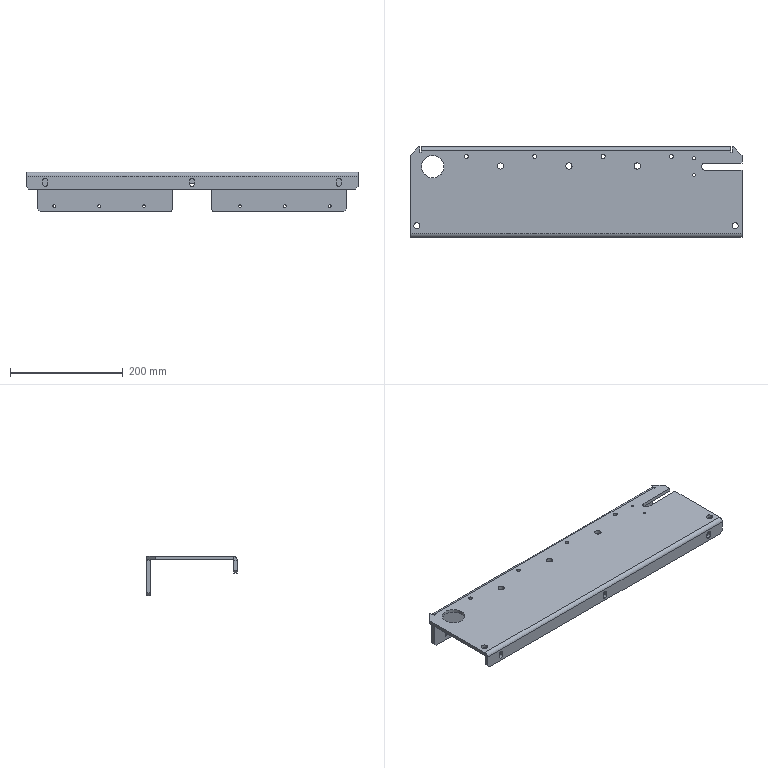Part | SolidWorks | features BaseBody 1 | 1 solid | 99 faces | box 588 x 160 x 70 mm | volume 806197 mm3 | cylinder 54 | plane 45 | commonest cylinder face diameters 5 x16 11 x10 9 x9 7 x8 10 x4 1.473 x2